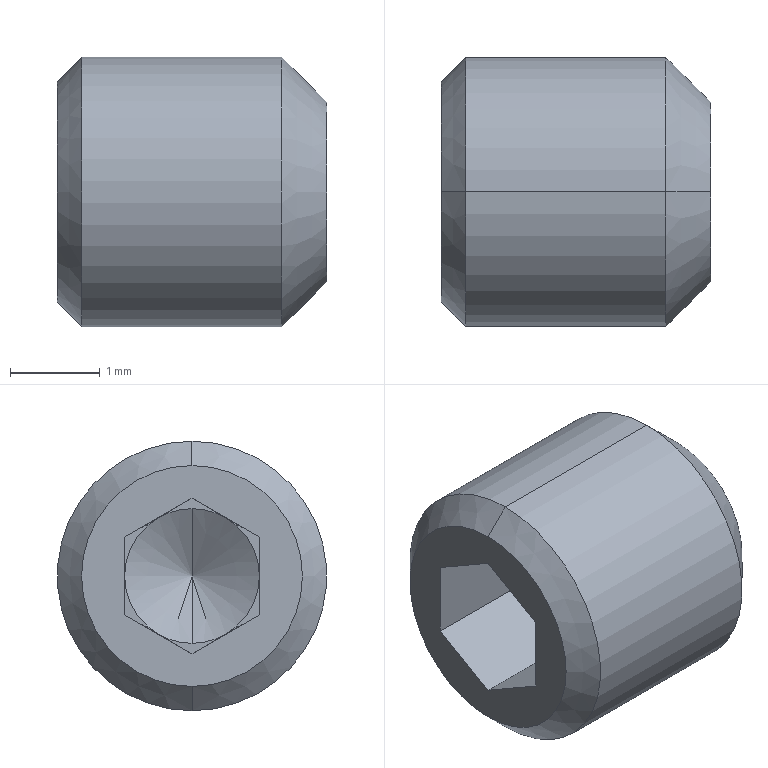Part | STEP file | Headless hex socket screw Dongming full thread M3-3 A2-70-1 | 1 solid | 22 faces | box 3 x 3 x 3 mm | volume 17.241 mm3 | plane 14 | cone 6 | cylinder 2 | commonest cylinder face diameters 3 x2
STEP:
#1=CARTESIAN_POINT('',(2.5,0.,1.5));
#2=VERTEX_POINT('',#1);
#3=CARTESIAN_POINT('',(2.5,0.,-1.5));
#4=VERTEX_POINT('',#3);
#5=CARTESIAN_POINT('',(2.5,0.,0.));
#6=DIRECTION('',(-1.,0.,0.));
#7=DIRECTION('',(0.,0.,1.));
#8=AXIS2_PLACEMENT_3D('',#5,#6,#7);
#9=CIRCLE('',#8,1.5);
#10=EDGE_CURVE('',#2,#4,#9,.T.);
#11=ORIENTED_EDGE('',*,*,#10,.T.);
#12=CARTESIAN_POINT('',(0.2705,0.,-1.5));
#13=VERTEX_POINT('',#12);
#14=CARTESIAN_POINT('',(-10.745,0.,-1.5));
#15=DIRECTION('',(-1.,0.,0.));
#16=VECTOR('',#15,1000.);
#17=LINE('',#14,#16);
#18=EDGE_CURVE('',#4,#13,#17,.T.);
#19=ORIENTED_EDGE('',*,*,#18,.T.);
#20=CARTESIAN_POINT('',(0.2705,0.,1.5));
#21=VERTEX_POINT('',#20);
#22=CARTESIAN_POINT('',(0.2705,0.,0.));
#23=DIRECTION('',(1.,0.,0.));
#24=DIRECTION('',(0.,0.,1.));
#25=AXIS2_PLACEMENT_3D('',#22,#23,#24);
#26=CIRCLE('',#25,1.5);
#27=EDGE_CURVE('',#13,#21,#26,.T.);
#28=ORIENTED_EDGE('',*,*,#27,.T.);
#29=CARTESIAN_POINT('',(-10.745,0.,1.5));
#30=DIRECTION('',(-1.,0.,0.));
#31=VECTOR('',#30,1000.);
#32=LINE('',#29,#31);
#33=EDGE_CURVE('',#2,#21,#32,.T.);
#34=ORIENTED_EDGE('',*,*,#33,.F.);
#35=EDGE_LOOP('',(#11,#19,#28,#34));
#36=FACE_OUTER_BOUND('',#35,.T.);
#37=CARTESIAN_POINT('',(-10.745,0.,0.));
#38=DIRECTION('',(-1.,0.,0.));
#39=DIRECTION('',(0.,0.,1.));
#40=AXIS2_PLACEMENT_3D('',#37,#38,#39);
#41=CYLINDRICAL_SURFACE('',#40,1.5);
#42=ADVANCED_FACE('',(#36),#41,.T.);
#43=CARTESIAN_POINT('',(0.,0.,-1.23));
#44=VERTEX_POINT('',#43);
#45=CARTESIAN_POINT('',(0.,0.,1.23));
#46=VERTEX_POINT('',#45);
#47=CARTESIAN_POINT('',(0.,0.,0.));
#48=DIRECTION('',(1.,0.,0.));
#49=DIRECTION('',(0.,0.,-1.));
#50=AXIS2_PLACEMENT_3D('',#47,#48,#49);
#51=CIRCLE('',#50,1.23);
#52=EDGE_CURVE('',#44,#46,#51,.T.);
#53=ORIENTED_EDGE('',*,*,#52,.T.);
#54=CARTESIAN_POINT('',(0.2705,0.,1.5));
#55=DIRECTION('',(0.7071,0.,0.7071));
#56=VECTOR('',#55,1000.);
#57=LINE('',#54,#56);
#58=EDGE_CURVE('',#46,#21,#57,.T.);
#59=ORIENTED_EDGE('',*,*,#58,.T.);
#60=ORIENTED_EDGE('',*,*,#27,.F.);
#61=CARTESIAN_POINT('',(0.2705,0.,-1.5));
#62=DIRECTION('',(0.7071,0.,-0.7071));
#63=VECTOR('',#62,1000.);
#64=LINE('',#61,#63);
#65=EDGE_CURVE('',#44,#13,#64,.T.);
#66=ORIENTED_EDGE('',*,*,#65,.F.);
#67=EDGE_LOOP('',(#53,#59,#60,#66));
#68=FACE_OUTER_BOUND('',#67,.T.);
#69=CARTESIAN_POINT('',(0.2705,0.,0.));
#70=DIRECTION('',(1.,0.,0.));
#71=DIRECTION('',(0.,0.,-1.));
#72=AXIS2_PLACEMENT_3D('',#69,#70,#71);
#73=CONICAL_SURFACE('',#72,1.5,0.7854);
#74=ADVANCED_FACE('',(#68),#73,.T.);
#75=CARTESIAN_POINT('',(3.,0.,1.));
#76=VERTEX_POINT('',#75);
#77=CARTESIAN_POINT('',(3.,0.,-1.));
#78=VERTEX_POINT('',#77);
#79=CARTESIAN_POINT('',(3.,0.,0.));
#80=DIRECTION('',(-1.,0.,0.));
#81=DIRECTION('',(0.,0.,1.));
#82=AXIS2_PLACEMENT_3D('',#79,#80,#81);
#83=CIRCLE('',#82,1.);
#84=EDGE_CURVE('',#76,#78,#83,.T.);
#85=ORIENTED_EDGE('',*,*,#84,.T.);
#86=CARTESIAN_POINT('',(2.5,0.,-1.5));
#87=DIRECTION('',(-0.7071,0.,-0.7071));
#88=VECTOR('',#87,1000.);
#89=LINE('',#86,#88);
#90=EDGE_CURVE('',#78,#4,#89,.T.);
#91=ORIENTED_EDGE('',*,*,#90,.T.);
#92=ORIENTED_EDGE('',*,*,#10,.F.);
#93=CARTESIAN_POINT('',(2.5,0.,1.5));
#94=DIRECTION('',(-0.7071,0.,0.7071));
#95=VECTOR('',#94,1000.);
#96=LINE('',#93,#95);
#97=EDGE_CURVE('',#76,#2,#96,.T.);
#98=ORIENTED_EDGE('',*,*,#97,.F.);
#99=EDGE_LOOP('',(#85,#91,#92,#98));
#100=FACE_OUTER_BOUND('',#99,.T.);
#101=CARTESIAN_POINT('',(2.5,0.,0.));
#102=DIRECTION('',(-1.,0.,0.));
#103=DIRECTION('',(0.,0.,1.));
#104=AXIS2_PLACEMENT_3D('',#101,#102,#103);
#105=CONICAL_SURFACE('',#104,1.5,0.7854);
#106=ADVANCED_FACE('',(#100),#105,.T.);
#107=CARTESIAN_POINT('',(1.633,0.,0.));
#108=VERTEX_POINT('',#107);
#109=CARTESIAN_POINT('',(1.2,0.,0.75));
#110=VERTEX_POINT('',#109);
#111=CARTESIAN_POINT('',(1.2,0.,0.75));
#112=DIRECTION('',(-0.5,0.,0.866));
#113=VECTOR('',#112,1000.);
#114=LINE('',#111,#113);
#115=EDGE_CURVE('',#108,#110,#114,.T.);
#116=ORIENTED_EDGE('',*,*,#115,.F.);
#117=CARTESIAN_POINT('',(1.2,0.,-0.75));
#118=VERTEX_POINT('',#117);
#119=CARTESIAN_POINT('',(1.2,0.,-0.75));
#120=DIRECTION('',(-0.5,0.,-0.866));
#121=VECTOR('',#120,1000.);
#122=LINE('',#119,#121);
#123=EDGE_CURVE('',#108,#118,#122,.T.);
#124=ORIENTED_EDGE('',*,*,#123,.T.);
#125=CARTESIAN_POINT('',(1.2,-0.375,-0.6495));
#126=VERTEX_POINT('',#125);
#127=CARTESIAN_POINT('',(1.2,0.,0.));
#128=DIRECTION('',(1.,0.,0.));
#129=DIRECTION('',(0.,0.,1.));
#130=AXIS2_PLACEMENT_3D('',#127,#128,#129);
#131=CIRCLE('',#130,0.75);
#132=EDGE_CURVE('',#126,#118,#131,.T.);
#133=ORIENTED_EDGE('',*,*,#132,.F.);
#134=CARTESIAN_POINT('',(1.2,-0.75,0.));
#135=VERTEX_POINT('',#134);
#136=CARTESIAN_POINT('',(1.2,0.,0.));
#137=DIRECTION('',(1.,0.,0.));
#138=DIRECTION('',(0.,0.,1.));
#139=AXIS2_PLACEMENT_3D('',#136,#137,#138);
#140=CIRCLE('',#139,0.75);
#141=EDGE_CURVE('',#135,#126,#140,.T.);
#142=ORIENTED_EDGE('',*,*,#141,.F.);
#143=CARTESIAN_POINT('',(1.2,-0.375,0.6495));
#144=VERTEX_POINT('',#143);
#145=CARTESIAN_POINT('',(1.2,0.,0.));
#146=DIRECTION('',(1.,0.,0.));
#147=DIRECTION('',(0.,0.,1.));
#148=AXIS2_PLACEMENT_3D('',#145,#146,#147);
#149=CIRCLE('',#148,0.75);
#150=EDGE_CURVE('',#144,#135,#149,.T.);
#151=ORIENTED_EDGE('',*,*,#150,.F.);
#152=CARTESIAN_POINT('',(1.2,0.,0.));
#153=DIRECTION('',(1.,0.,0.));
#154=DIRECTION('',(0.,0.,1.));
#155=AXIS2_PLACEMENT_3D('',#152,#153,#154);
#156=CIRCLE('',#155,0.75);
#157=EDGE_CURVE('',#110,#144,#156,.T.);
#158=ORIENTED_EDGE('',*,*,#157,.F.);
#159=EDGE_LOOP('',(#116,#124,#133,#142,#151,#158));
#160=FACE_OUTER_BOUND('',#159,.T.);
#161=CARTESIAN_POINT('',(1.2,0.,0.));
#162=DIRECTION('',(-1.,0.,0.));
#163=DIRECTION('',(0.,0.,1.));
#164=AXIS2_PLACEMENT_3D('',#161,#162,#163);
#165=CONICAL_SURFACE('',#164,0.75,1.047);
#166=ADVANCED_FACE('',(#160),#165,.F.);
#167=ORIENTED_EDGE('',*,*,#18,.F.);
#168=CARTESIAN_POINT('',(2.5,0.,0.));
#169=DIRECTION('',(-1.,0.,0.));
#170=DIRECTION('',(0.,0.,1.));
#171=AXIS2_PLACEMENT_3D('',#168,#169,#170);
#172=CIRCLE('',#171,1.5);
#173=EDGE_CURVE('',#4,#2,#172,.T.);
#174=ORIENTED_EDGE('',*,*,#173,.T.);
#175=ORIENTED_EDGE('',*,*,#33,.T.);
#176=CARTESIAN_POINT('',(0.2705,0.,0.));
#177=DIRECTION('',(1.,0.,0.));
#178=DIRECTION('',(0.,0.,1.));
#179=AXIS2_PLACEMENT_3D('',#176,#177,#178);
#180=CIRCLE('',#179,1.5);
#181=EDGE_CURVE('',#21,#13,#180,.T.);
#182=ORIENTED_EDGE('',*,*,#181,.T.);
#183=EDGE_LOOP('',(#167,#174,#175,#182));
#184=FACE_OUTER_BOUND('',#183,.T.);
#185=CARTESIAN_POINT('',(-10.745,0.,0.));
#186=DIRECTION('',(-1.,0.,0.));
#187=DIRECTION('',(0.,0.,1.));
#188=AXIS2_PLACEMENT_3D('',#185,#186,#187);
#189=CYLINDRICAL_SURFACE('',#188,1.5);
#190=ADVANCED_FACE('',(#184),#189,.T.);
#191=ORIENTED_EDGE('',*,*,#58,.F.);
#192=CARTESIAN_POINT('',(0.,0.,0.));
#193=DIRECTION('',(1.,0.,0.));
#194=DIRECTION('',(0.,0.,-1.));
#195=AXIS2_PLACEMENT_3D('',#192,#193,#194);
#196=CIRCLE('',#195,1.23);
#197=EDGE_CURVE('',#46,#44,#196,.T.);
#198=ORIENTED_EDGE('',*,*,#197,.T.);
#199=ORIENTED_EDGE('',*,*,#65,.T.);
#200=ORIENTED_EDGE('',*,*,#181,.F.);
#201=EDGE_LOOP('',(#191,#198,#199,#200));
#202=FACE_OUTER_BOUND('',#201,.T.);
#203=CARTESIAN_POINT('',(0.2705,0.,0.));
#204=DIRECTION('',(1.,0.,0.));
#205=DIRECTION('',(0.,0.,-1.));
#206=AXIS2_PLACEMENT_3D('',#203,#204,#205);
#207=CONICAL_SURFACE('',#206,1.5,0.7854);
#208=ADVANCED_FACE('',(#202),#207,.T.);
#209=ORIENTED_EDGE('',*,*,#90,.F.);
#210=CARTESIAN_POINT('',(3.,0.,0.));
#211=DIRECTION('',(-1.,0.,0.));
#212=DIRECTION('',(0.,0.,1.));
#213=AXIS2_PLACEMENT_3D('',#210,#211,#212);
#214=CIRCLE('',#213,1.);
#215=EDGE_CURVE('',#78,#76,#214,.T.);
#216=ORIENTED_EDGE('',*,*,#215,.T.);
#217=ORIENTED_EDGE('',*,*,#97,.T.);
#218=ORIENTED_EDGE('',*,*,#173,.F.);
#219=EDGE_LOOP('',(#209,#216,#217,#218));
#220=FACE_OUTER_BOUND('',#219,.T.);
#221=CARTESIAN_POINT('',(2.5,0.,0.));
#222=DIRECTION('',(-1.,0.,0.));
#223=DIRECTION('',(0.,0.,1.));
#224=AXIS2_PLACEMENT_3D('',#221,#222,#223);
#225=CONICAL_SURFACE('',#224,1.5,0.7854);
#226=ADVANCED_FACE('',(#220),#225,.T.);
#227=ORIENTED_EDGE('',*,*,#52,.F.);
#228=ORIENTED_EDGE('',*,*,#197,.F.);
#229=EDGE_LOOP('',(#227,#228));
#230=FACE_OUTER_BOUND('',#229,.T.);
#231=CARTESIAN_POINT('',(0.,-0.75,0.433));
#232=VERTEX_POINT('',#231);
#233=CARTESIAN_POINT('',(0.,0.,0.866));
#234=VERTEX_POINT('',#233);
#235=CARTESIAN_POINT('',(0.,-0.75,0.433));
#236=DIRECTION('',(0.,0.866,0.5));
#237=VECTOR('',#236,1000.);
#238=LINE('',#235,#237);
#239=EDGE_CURVE('',#232,#234,#238,.T.);
#240=ORIENTED_EDGE('',*,*,#239,.F.);
#241=CARTESIAN_POINT('',(0.,-0.75,-0.433));
#242=VERTEX_POINT('',#241);
#243=CARTESIAN_POINT('',(0.,-0.75,0.));
#244=DIRECTION('',(0.,0.,1.));
#245=VECTOR('',#244,1000.);
#246=LINE('',#243,#245);
#247=EDGE_CURVE('',#242,#232,#246,.T.);
#248=ORIENTED_EDGE('',*,*,#247,.F.);
#249=CARTESIAN_POINT('',(0.,0.,-0.866));
#250=VERTEX_POINT('',#249);
#251=CARTESIAN_POINT('',(0.,0.,-0.866));
#252=DIRECTION('',(0.,-0.866,0.5));
#253=VECTOR('',#252,1000.);
#254=LINE('',#251,#253);
#255=EDGE_CURVE('',#250,#242,#254,.T.);
#256=ORIENTED_EDGE('',*,*,#255,.F.);
#257=CARTESIAN_POINT('',(0.,0.75,-0.433));
#258=VERTEX_POINT('',#257);
#259=CARTESIAN_POINT('',(0.,0.75,-0.433));
#260=DIRECTION('',(0.,-0.866,-0.5));
#261=VECTOR('',#260,1000.);
#262=LINE('',#259,#261);
#263=EDGE_CURVE('',#258,#250,#262,.T.);
#264=ORIENTED_EDGE('',*,*,#263,.F.);
#265=CARTESIAN_POINT('',(0.,0.75,0.433));
#266=VERTEX_POINT('',#265);
#267=CARTESIAN_POINT('',(0.,0.75,0.));
#268=DIRECTION('',(0.,0.,-1.));
#269=VECTOR('',#268,1000.);
#270=LINE('',#267,#269);
#271=EDGE_CURVE('',#266,#258,#270,.T.);
#272=ORIENTED_EDGE('',*,*,#271,.F.);
#273=CARTESIAN_POINT('',(0.,0.,0.866));
#274=DIRECTION('',(0.,0.866,-0.5));
#275=VECTOR('',#274,1000.);
#276=LINE('',#273,#275);
#277=EDGE_CURVE('',#234,#266,#276,.T.);
#278=ORIENTED_EDGE('',*,*,#277,.F.);
#279=EDGE_LOOP('',(#240,#248,#256,#264,#272,#278));
#280=FACE_BOUND('',#279,.T.);
#281=CARTESIAN_POINT('',(0.,1.229,0.));
#282=DIRECTION('',(1.,0.,0.));
#283=DIRECTION('',(0.,0.,-1.));
#284=AXIS2_PLACEMENT_3D('',#281,#282,#283);
#285=PLANE('',#284);
#286=ADVANCED_FACE('',(#230,#280),#285,.F.);
#287=ORIENTED_EDGE('',*,*,#84,.F.);
#288=ORIENTED_EDGE('',*,*,#215,.F.);
#289=EDGE_LOOP('',(#287,#288));
#290=FACE_OUTER_BOUND('',#289,.T.);
#291=CARTESIAN_POINT('',(3.,0.,0.));
#292=DIRECTION('',(-1.,0.,0.));
#293=DIRECTION('',(0.,0.,1.));
#294=AXIS2_PLACEMENT_3D('',#291,#292,#293);
#295=PLANE('',#294);
#296=ADVANCED_FACE('',(#290),#295,.F.);
#297=CARTESIAN_POINT('',(1.2,0.75,0.433));
#298=VERTEX_POINT('',#297);
#299=CARTESIAN_POINT('',(1.2,0.75,0.433));
#300=DIRECTION('',(-1.,0.,0.));
#301=VECTOR('',#300,1000.);
#302=LINE('',#299,#301);
#303=EDGE_CURVE('',#298,#266,#302,.T.);
#304=ORIENTED_EDGE('',*,*,#303,.F.);
#305=CARTESIAN_POINT('',(1.2,0.375,0.6495));
#306=VERTEX_POINT('',#305);
#307=CARTESIAN_POINT('',(1.2,0.,0.866));
#308=DIRECTION('',(0.,0.866,-0.5));
#309=VECTOR('',#308,1000.);
#310=LINE('',#307,#309);
#311=EDGE_CURVE('',#306,#298,#310,.T.);
#312=ORIENTED_EDGE('',*,*,#311,.F.);
#313=CARTESIAN_POINT('',(1.2,0.,0.866));
#314=VERTEX_POINT('',#313);
#315=CARTESIAN_POINT('',(1.2,0.,0.866));
#316=DIRECTION('',(0.,0.866,-0.5));
#317=VECTOR('',#316,1000.);
#318=LINE('',#315,#317);
#319=EDGE_CURVE('',#314,#306,#318,.T.);
#320=ORIENTED_EDGE('',*,*,#319,.F.);
#321=CARTESIAN_POINT('',(1.2,0.,0.866));
#322=DIRECTION('',(1.,0.,0.));
#323=VECTOR('',#322,1000.);
#324=LINE('',#321,#323);
#325=EDGE_CURVE('',#234,#314,#324,.T.);
#326=ORIENTED_EDGE('',*,*,#325,.F.);
#327=ORIENTED_EDGE('',*,*,#277,.T.);
#328=EDGE_LOOP('',(#304,#312,#320,#326,#327));
#329=FACE_OUTER_BOUND('',#328,.T.);
#330=CARTESIAN_POINT('',(1.2,0.,0.866));
#331=DIRECTION('',(0.,0.5,0.866));
#332=DIRECTION('',(0.,-0.866,0.5));
#333=AXIS2_PLACEMENT_3D('',#330,#331,#332);
#334=PLANE('',#333);
#335=ADVANCED_FACE('',(#329),#334,.F.);
#336=ORIENTED_EDGE('',*,*,#325,.T.);
#337=CARTESIAN_POINT('',(1.2,-0.75,0.433));
#338=DIRECTION('',(0.,0.866,0.5));
#339=VECTOR('',#338,1000.);
#340=LINE('',#337,#339);
#341=EDGE_CURVE('',#144,#314,#340,.T.);
#342=ORIENTED_EDGE('',*,*,#341,.F.);
#343=CARTESIAN_POINT('',(1.2,-0.75,0.433));
#344=VERTEX_POINT('',#343);
#345=CARTESIAN_POINT('',(1.2,-0.75,0.433));
#346=DIRECTION('',(0.,0.866,0.5));
#347=VECTOR('',#346,1000.);
#348=LINE('',#345,#347);
#349=EDGE_CURVE('',#344,#144,#348,.T.);
#350=ORIENTED_EDGE('',*,*,#349,.F.);
#351=CARTESIAN_POINT('',(1.2,-0.75,0.433));
#352=DIRECTION('',(1.,0.,0.));
#353=VECTOR('',#352,1000.);
#354=LINE('',#351,#353);
#355=EDGE_CURVE('',#232,#344,#354,.T.);
#356=ORIENTED_EDGE('',*,*,#355,.F.);
#357=ORIENTED_EDGE('',*,*,#239,.T.);
#358=EDGE_LOOP('',(#336,#342,#350,#356,#357));
#359=FACE_OUTER_BOUND('',#358,.T.);
#360=CARTESIAN_POINT('',(1.2,-0.75,0.433));
#361=DIRECTION('',(0.,-0.5,0.866));
#362=DIRECTION('',(0.,-0.866,-0.5));
#363=AXIS2_PLACEMENT_3D('',#360,#361,#362);
#364=PLANE('',#363);
#365=ADVANCED_FACE('',(#359),#364,.F.);
#366=ORIENTED_EDGE('',*,*,#355,.T.);
#367=CARTESIAN_POINT('',(1.2,-0.75,-0.433));
#368=DIRECTION('',(0.,0.,1.));
#369=VECTOR('',#368,1000.);
#370=LINE('',#367,#369);
#371=EDGE_CURVE('',#135,#344,#370,.T.);
#372=ORIENTED_EDGE('',*,*,#371,.F.);
#373=CARTESIAN_POINT('',(1.2,-0.75,-0.433));
#374=VERTEX_POINT('',#373);
#375=CARTESIAN_POINT('',(1.2,-0.75,-0.433));
#376=DIRECTION('',(0.,0.,1.));
#377=VECTOR('',#376,1000.);
#378=LINE('',#375,#377);
#379=EDGE_CURVE('',#374,#135,#378,.T.);
#380=ORIENTED_EDGE('',*,*,#379,.F.);
#381=CARTESIAN_POINT('',(1.2,-0.75,-0.433));
#382=DIRECTION('',(1.,0.,0.));
#383=VECTOR('',#382,1000.);
#384=LINE('',#381,#383);
#385=EDGE_CURVE('',#242,#374,#384,.T.);
#386=ORIENTED_EDGE('',*,*,#385,.F.);
#387=ORIENTED_EDGE('',*,*,#247,.T.);
#388=EDGE_LOOP('',(#366,#372,#380,#386,#387));
#389=FACE_OUTER_BOUND('',#388,.T.);
#390=CARTESIAN_POINT('',(1.2,-0.75,-0.433));
#391=DIRECTION('',(0.,-1.,0.));
#392=DIRECTION('',(0.,0.,-1.));
#393=AXIS2_PLACEMENT_3D('',#390,#391,#392);
#394=PLANE('',#393);
#395=ADVANCED_FACE('',(#389),#394,.F.);
#396=ORIENTED_EDGE('',*,*,#385,.T.);
#397=CARTESIAN_POINT('',(1.2,0.,-0.866));
#398=DIRECTION('',(0.,-0.866,0.5));
#399=VECTOR('',#398,1000.);
#400=LINE('',#397,#399);
#401=EDGE_CURVE('',#126,#374,#400,.T.);
#402=ORIENTED_EDGE('',*,*,#401,.F.);
#403=CARTESIAN_POINT('',(1.2,0.,-0.866));
#404=VERTEX_POINT('',#403);
#405=CARTESIAN_POINT('',(1.2,0.,-0.866));
#406=DIRECTION('',(0.,-0.866,0.5));
#407=VECTOR('',#406,1000.);
#408=LINE('',#405,#407);
#409=EDGE_CURVE('',#404,#126,#408,.T.);
#410=ORIENTED_EDGE('',*,*,#409,.F.);
#411=CARTESIAN_POINT('',(1.2,0.,-0.866));
#412=DIRECTION('',(1.,0.,0.));
#413=VECTOR('',#412,1000.);
#414=LINE('',#411,#413);
#415=EDGE_CURVE('',#250,#404,#414,.T.);
#416=ORIENTED_EDGE('',*,*,#415,.F.);
#417=ORIENTED_EDGE('',*,*,#255,.T.);
#418=EDGE_LOOP('',(#396,#402,#410,#416,#417));
#419=FACE_OUTER_BOUND('',#418,.T.);
#420=CARTESIAN_POINT('',(1.2,0.,-0.866));
#421=DIRECTION('',(0.,-0.5,-0.866));
#422=DIRECTION('',(0.,0.866,-0.5));
#423=AXIS2_PLACEMENT_3D('',#420,#421,#422);
#424=PLANE('',#423);
#425=ADVANCED_FACE('',(#419),#424,.F.);
#426=ORIENTED_EDGE('',*,*,#415,.T.);
#427=CARTESIAN_POINT('',(1.2,0.375,-0.6495));
#428=VERTEX_POINT('',#427);
#429=CARTESIAN_POINT('',(1.2,0.75,-0.433));
#430=DIRECTION('',(0.,-0.866,-0.5));
#431=VECTOR('',#430,1000.);
#432=LINE('',#429,#431);
#433=EDGE_CURVE('',#428,#404,#432,.T.);
#434=ORIENTED_EDGE('',*,*,#433,.F.);
#435=CARTESIAN_POINT('',(1.2,0.75,-0.433));
#436=VERTEX_POINT('',#435);
#437=CARTESIAN_POINT('',(1.2,0.75,-0.433));
#438=DIRECTION('',(0.,-0.866,-0.5));
#439=VECTOR('',#438,1000.);
#440=LINE('',#437,#439);
#441=EDGE_CURVE('',#436,#428,#440,.T.);
#442=ORIENTED_EDGE('',*,*,#441,.F.);
#443=CARTESIAN_POINT('',(1.2,0.75,-0.433));
#444=DIRECTION('',(1.,0.,0.));
#445=VECTOR('',#444,1000.);
#446=LINE('',#443,#445);
#447=EDGE_CURVE('',#258,#436,#446,.T.);
#448=ORIENTED_EDGE('',*,*,#447,.F.);
#449=ORIENTED_EDGE('',*,*,#263,.T.);
#450=EDGE_LOOP('',(#426,#434,#442,#448,#449));
#451=FACE_OUTER_BOUND('',#450,.T.);
#452=CARTESIAN_POINT('',(1.2,0.75,-0.433));
#453=DIRECTION('',(0.,0.5,-0.866));
#454=DIRECTION('',(0.,0.866,0.5));
#455=AXIS2_PLACEMENT_3D('',#452,#453,#454);
#456=PLANE('',#455);
#457=ADVANCED_FACE('',(#451),#456,.F.);
#458=ORIENTED_EDGE('',*,*,#447,.T.);
#459=CARTESIAN_POINT('',(1.2,0.75,0.));
#460=VERTEX_POINT('',#459);
#461=CARTESIAN_POINT('',(1.2,0.75,0.433));
#462=DIRECTION('',(0.,0.,-1.));
#463=VECTOR('',#462,1000.);
#464=LINE('',#461,#463);
#465=EDGE_CURVE('',#460,#436,#464,.T.);
#466=ORIENTED_EDGE('',*,*,#465,.F.);
#467=CARTESIAN_POINT('',(1.2,0.75,0.433));
#468=DIRECTION('',(0.,0.,-1.));
#469=VECTOR('',#468,1000.);
#470=LINE('',#467,#469);
#471=EDGE_CURVE('',#298,#460,#470,.T.);
#472=ORIENTED_EDGE('',*,*,#471,.F.);
#473=ORIENTED_EDGE('',*,*,#303,.T.);
#474=ORIENTED_EDGE('',*,*,#271,.T.);
#475=EDGE_LOOP('',(#458,#466,#472,#473,#474));
#476=FACE_OUTER_BOUND('',#475,.T.);
#477=CARTESIAN_POINT('',(1.2,0.75,0.433));
#478=DIRECTION('',(0.,1.,0.));
#479=DIRECTION('',(0.,0.,1.));
#480=AXIS2_PLACEMENT_3D('',#477,#478,#479);
#481=PLANE('',#480);
#482=ADVANCED_FACE('',(#476),#481,.F.);
#483=ORIENTED_EDGE('',*,*,#311,.T.);
#484=ORIENTED_EDGE('',*,*,#471,.T.);
#485=CARTESIAN_POINT('',(1.2,0.,0.));
#486=DIRECTION('',(1.,0.,0.));
#487=DIRECTION('',(0.,0.,1.));
#488=AXIS2_PLACEMENT_3D('',#485,#486,#487);
#489=CIRCLE('',#488,0.75);
#490=EDGE_CURVE('',#460,#306,#489,.T.);
#491=ORIENTED_EDGE('',*,*,#490,.T.);
#492=EDGE_LOOP('',(#483,#484,#491));
#493=FACE_OUTER_BOUND('',#492,.T.);
#494=CARTESIAN_POINT('',(1.2,0.,0.866));
#495=DIRECTION('',(-1.,0.,0.));
#496=DIRECTION('',(0.,0.,1.));
#497=AXIS2_PLACEMENT_3D('',#494,#495,#496);
#498=PLANE('',#497);
#499=ADVANCED_FACE('',(#493),#498,.T.);
#500=ORIENTED_EDGE('',*,*,#319,.T.);
#501=CARTESIAN_POINT('',(1.2,0.,0.));
#502=DIRECTION('',(1.,0.,0.));
#503=DIRECTION('',(0.,0.,1.));
#504=AXIS2_PLACEMENT_3D('',#501,#502,#503);
#505=CIRCLE('',#504,0.75);
#506=EDGE_CURVE('',#306,#110,#505,.T.);
#507=ORIENTED_EDGE('',*,*,#506,.T.);
#508=ORIENTED_EDGE('',*,*,#157,.T.);
#509=ORIENTED_EDGE('',*,*,#341,.T.);
#510=EDGE_LOOP('',(#500,#507,#508,#509));
#511=FACE_OUTER_BOUND('',#510,.T.);
#512=CARTESIAN_POINT('',(1.2,0.,0.866));
#513=DIRECTION('',(-1.,0.,0.));
#514=DIRECTION('',(0.,0.,1.));
#515=AXIS2_PLACEMENT_3D('',#512,#513,#514);
#516=PLANE('',#515);
#517=ADVANCED_FACE('',(#511),#516,.T.);
#518=ORIENTED_EDGE('',*,*,#371,.T.);
#519=ORIENTED_EDGE('',*,*,#349,.T.);
#520=ORIENTED_EDGE('',*,*,#150,.T.);
#521=EDGE_LOOP('',(#518,#519,#520));
#522=FACE_OUTER_BOUND('',#521,.T.);
#523=CARTESIAN_POINT('',(1.2,0.,0.866));
#524=DIRECTION('',(-1.,0.,0.));
#525=DIRECTION('',(0.,0.,1.));
#526=AXIS2_PLACEMENT_3D('',#523,#524,#525);
#527=PLANE('',#526);
#528=ADVANCED_FACE('',(#522),#527,.T.);
#529=ORIENTED_EDGE('',*,*,#401,.T.);
#530=ORIENTED_EDGE('',*,*,#379,.T.);
#531=ORIENTED_EDGE('',*,*,#141,.T.);
#532=EDGE_LOOP('',(#529,#530,#531));
#533=FACE_OUTER_BOUND('',#532,.T.);
#534=CARTESIAN_POINT('',(1.2,0.,0.866));
#535=DIRECTION('',(-1.,0.,0.));
#536=DIRECTION('',(0.,0.,1.));
#537=AXIS2_PLACEMENT_3D('',#534,#535,#536);
#538=PLANE('',#537);
#539=ADVANCED_FACE('',(#533),#538,.T.);
#540=ORIENTED_EDGE('',*,*,#409,.T.);
#541=ORIENTED_EDGE('',*,*,#132,.T.);
#542=CARTESIAN_POINT('',(1.2,0.,0.));
#543=DIRECTION('',(1.,0.,0.));
#544=DIRECTION('',(0.,0.,1.));
#545=AXIS2_PLACEMENT_3D('',#542,#543,#544);
#546=CIRCLE('',#545,0.75);
#547=EDGE_CURVE('',#118,#428,#546,.T.);
#548=ORIENTED_EDGE('',*,*,#547,.T.);
#549=ORIENTED_EDGE('',*,*,#433,.T.);
#550=EDGE_LOOP('',(#540,#541,#548,#549));
#551=FACE_OUTER_BOUND('',#550,.T.);
#552=CARTESIAN_POINT('',(1.2,0.,0.866));
#553=DIRECTION('',(-1.,0.,0.));
#554=DIRECTION('',(0.,0.,1.));
#555=AXIS2_PLACEMENT_3D('',#552,#553,#554);
#556=PLANE('',#555);
#557=ADVANCED_FACE('',(#551),#556,.T.);
#558=ORIENTED_EDGE('',*,*,#465,.T.);
#559=ORIENTED_EDGE('',*,*,#441,.T.);
#560=CARTESIAN_POINT('',(1.2,0.,0.));
#561=DIRECTION('',(1.,0.,0.));
#562=DIRECTION('',(0.,0.,1.));
#563=AXIS2_PLACEMENT_3D('',#560,#561,#562);
#564=CIRCLE('',#563,0.75);
#565=EDGE_CURVE('',#428,#460,#564,.T.);
#566=ORIENTED_EDGE('',*,*,#565,.T.);
#567=EDGE_LOOP('',(#558,#559,#566));
#568=FACE_OUTER_BOUND('',#567,.T.);
#569=CARTESIAN_POINT('',(1.2,0.,0.866));
#570=DIRECTION('',(-1.,0.,0.));
#571=DIRECTION('',(0.,0.,1.));
#572=AXIS2_PLACEMENT_3D('',#569,#570,#571);
#573=PLANE('',#572);
#574=ADVANCED_FACE('',(#568),#573,.T.);
#575=ORIENTED_EDGE('',*,*,#123,.F.);
#576=ORIENTED_EDGE('',*,*,#115,.T.);
#577=ORIENTED_EDGE('',*,*,#506,.F.);
#578=ORIENTED_EDGE('',*,*,#490,.F.);
#579=ORIENTED_EDGE('',*,*,#565,.F.);
#580=ORIENTED_EDGE('',*,*,#547,.F.);
#581=EDGE_LOOP('',(#575,#576,#577,#578,#579,#580));
#582=FACE_OUTER_BOUND('',#581,.T.);
#583=CARTESIAN_POINT('',(1.2,0.,0.));
#584=DIRECTION('',(-1.,0.,0.));
#585=DIRECTION('',(0.,0.,1.));
#586=AXIS2_PLACEMENT_3D('',#583,#584,#585);
#587=CONICAL_SURFACE('',#586,0.75,1.047);
#588=ADVANCED_FACE('',(#582),#587,.F.);
#589=CLOSED_SHELL('',(#42,#74,#106,#166,#190,#208,#226,#286,#296,#335,#365,#395,#425,#457,#482,#499,#517,#528,#539,#557,#574,#588));
#590=MANIFOLD_SOLID_BREP('',#589);
#591=CARTESIAN_POINT('',(0.,0.,0.));
#592=DIRECTION('',(0.,0.,1.));
#593=DIRECTION('',(1.,0.,0.));
#594=AXIS2_PLACEMENT_3D('',#591,#592,#593);
#595=(LENGTH_UNIT()NAMED_UNIT(*)SI_UNIT(.MILLI.,.METRE.));
#596=UNCERTAINTY_MEASURE_WITH_UNIT(LENGTH_MEASURE(0.00001),#595,'','');
#597=(NAMED_UNIT(*)PLANE_ANGLE_UNIT()SI_UNIT($,.RADIAN.));
#598=(NAMED_UNIT(*)SI_UNIT($,.STERADIAN.)SOLID_ANGLE_UNIT());
#599=(GEOMETRIC_REPRESENTATION_CONTEXT(3)GLOBAL_UNCERTAINTY_ASSIGNED_CONTEXT((#596))GLOBAL_UNIT_ASSIGNED_CONTEXT((#595,#597,#598))REPRESENTATION_CONTEXT('',''));
#600=ADVANCED_BREP_SHAPE_REPRESENTATION('',(#590,#594),#599);